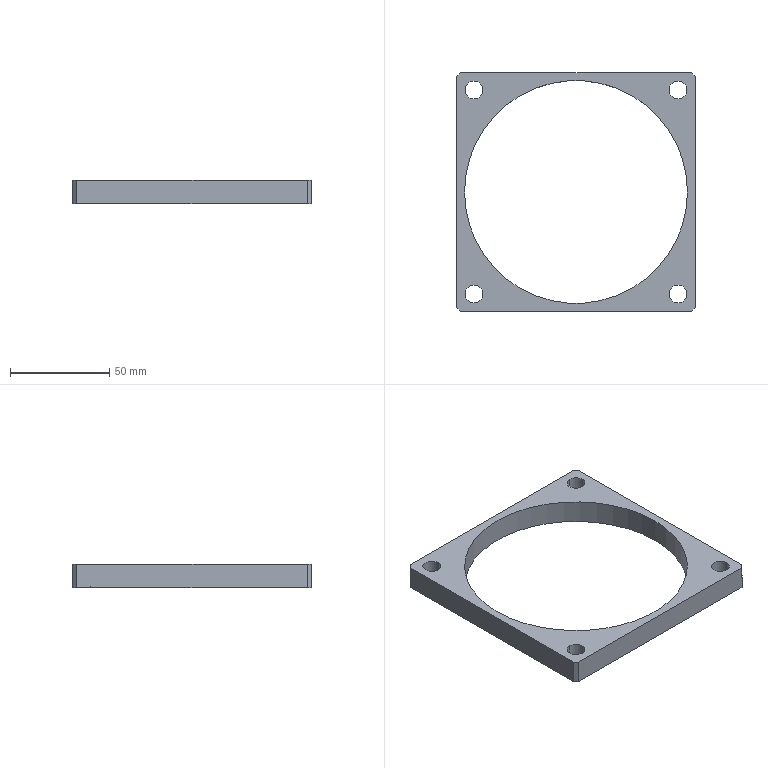Part | SolidWorks | features Chamfer 1, CirPattern 1, Extrusion 1, HoleWzd 1, ICE 1 | 1 solid | 20 faces | box 120 x 120 x 12 mm | volume 51426 mm3 | cylinder 10 | plane 10 | commonest cylinder face diameters 9 x8 112 x2
STEP:
#1=CARTESIAN_POINT('',(51.265,55.765,0.));
#2=VERTEX_POINT('',#1);
#3=CARTESIAN_POINT('',(51.265,46.765,0.));
#4=VERTEX_POINT('',#3);
#5=CARTESIAN_POINT('',(51.265,51.265,0.));
#6=DIRECTION('',(0.,0.,1.));
#7=DIRECTION('',(0.,-1.,0.));
#8=AXIS2_PLACEMENT_3D('',#5,#6,#7);
#9=CIRCLE('',#8,4.5);
#10=EDGE_CURVE('',#2,#4,#9,.T.);
#11=ORIENTED_EDGE('',*,*,#10,.F.);
#12=CARTESIAN_POINT('',(51.265,55.765,12.));
#13=VERTEX_POINT('',#12);
#14=CARTESIAN_POINT('',(51.265,55.765,12.));
#15=DIRECTION('',(0.,0.,1.));
#16=VECTOR('',#15,1000.);
#17=LINE('',#14,#16);
#18=EDGE_CURVE('',#2,#13,#17,.T.);
#19=ORIENTED_EDGE('',*,*,#18,.T.);
#20=CARTESIAN_POINT('',(51.265,46.765,12.));
#21=VERTEX_POINT('',#20);
#22=CARTESIAN_POINT('',(51.265,51.265,12.));
#23=DIRECTION('',(0.,0.,1.));
#24=DIRECTION('',(0.,-1.,0.));
#25=AXIS2_PLACEMENT_3D('',#22,#23,#24);
#26=CIRCLE('',#25,4.5);
#27=EDGE_CURVE('',#13,#21,#26,.T.);
#28=ORIENTED_EDGE('',*,*,#27,.T.);
#29=CARTESIAN_POINT('',(51.265,46.765,12.));
#30=DIRECTION('',(0.,0.,1.));
#31=VECTOR('',#30,1000.);
#32=LINE('',#29,#31);
#33=EDGE_CURVE('',#4,#21,#32,.T.);
#34=ORIENTED_EDGE('',*,*,#33,.F.);
#35=EDGE_LOOP('',(#11,#19,#28,#34));
#36=FACE_OUTER_BOUND('',#35,.T.);
#37=CARTESIAN_POINT('',(51.265,51.265,12.));
#38=DIRECTION('',(0.,0.,1.));
#39=DIRECTION('',(0.,-1.,0.));
#40=AXIS2_PLACEMENT_3D('',#37,#38,#39);
#41=CYLINDRICAL_SURFACE('',#40,4.5);
#42=ADVANCED_FACE('',(#36),#41,.F.);
#43=CARTESIAN_POINT('',(55.765,-51.265,0.));
#44=VERTEX_POINT('',#43);
#45=CARTESIAN_POINT('',(46.765,-51.265,0.));
#46=VERTEX_POINT('',#45);
#47=CARTESIAN_POINT('',(51.265,-51.265,0.));
#48=DIRECTION('',(0.,0.,1.));
#49=DIRECTION('',(-1.,0.,0.));
#50=AXIS2_PLACEMENT_3D('',#47,#48,#49);
#51=CIRCLE('',#50,4.5);
#52=EDGE_CURVE('',#44,#46,#51,.T.);
#53=ORIENTED_EDGE('',*,*,#52,.F.);
#54=CARTESIAN_POINT('',(55.765,-51.265,12.));
#55=VERTEX_POINT('',#54);
#56=CARTESIAN_POINT('',(55.765,-51.265,12.));
#57=DIRECTION('',(0.,0.,1.));
#58=VECTOR('',#57,1000.);
#59=LINE('',#56,#58);
#60=EDGE_CURVE('',#44,#55,#59,.T.);
#61=ORIENTED_EDGE('',*,*,#60,.T.);
#62=CARTESIAN_POINT('',(46.765,-51.265,12.));
#63=VERTEX_POINT('',#62);
#64=CARTESIAN_POINT('',(51.265,-51.265,12.));
#65=DIRECTION('',(0.,0.,1.));
#66=DIRECTION('',(-1.,0.,0.));
#67=AXIS2_PLACEMENT_3D('',#64,#65,#66);
#68=CIRCLE('',#67,4.5);
#69=EDGE_CURVE('',#55,#63,#68,.T.);
#70=ORIENTED_EDGE('',*,*,#69,.T.);
#71=CARTESIAN_POINT('',(46.765,-51.265,12.));
#72=DIRECTION('',(0.,0.,1.));
#73=VECTOR('',#72,1000.);
#74=LINE('',#71,#73);
#75=EDGE_CURVE('',#46,#63,#74,.T.);
#76=ORIENTED_EDGE('',*,*,#75,.F.);
#77=EDGE_LOOP('',(#53,#61,#70,#76));
#78=FACE_OUTER_BOUND('',#77,.T.);
#79=CARTESIAN_POINT('',(51.265,-51.265,12.));
#80=DIRECTION('',(0.,0.,1.));
#81=DIRECTION('',(-1.,0.,0.));
#82=AXIS2_PLACEMENT_3D('',#79,#80,#81);
#83=CYLINDRICAL_SURFACE('',#82,4.5);
#84=ADVANCED_FACE('',(#78),#83,.F.);
#85=CARTESIAN_POINT('',(-51.265,-55.765,0.));
#86=VERTEX_POINT('',#85);
#87=CARTESIAN_POINT('',(-51.265,-46.765,0.));
#88=VERTEX_POINT('',#87);
#89=CARTESIAN_POINT('',(-51.265,-51.265,0.));
#90=DIRECTION('',(0.,0.,1.));
#91=DIRECTION('',(0.,1.,0.));
#92=AXIS2_PLACEMENT_3D('',#89,#90,#91);
#93=CIRCLE('',#92,4.5);
#94=EDGE_CURVE('',#86,#88,#93,.T.);
#95=ORIENTED_EDGE('',*,*,#94,.F.);
#96=CARTESIAN_POINT('',(-51.265,-55.765,12.));
#97=VERTEX_POINT('',#96);
#98=CARTESIAN_POINT('',(-51.265,-55.765,12.));
#99=DIRECTION('',(0.,0.,1.));
#100=VECTOR('',#99,1000.);
#101=LINE('',#98,#100);
#102=EDGE_CURVE('',#86,#97,#101,.T.);
#103=ORIENTED_EDGE('',*,*,#102,.T.);
#104=CARTESIAN_POINT('',(-51.265,-46.765,12.));
#105=VERTEX_POINT('',#104);
#106=CARTESIAN_POINT('',(-51.265,-51.265,12.));
#107=DIRECTION('',(0.,0.,1.));
#108=DIRECTION('',(0.,1.,0.));
#109=AXIS2_PLACEMENT_3D('',#106,#107,#108);
#110=CIRCLE('',#109,4.5);
#111=EDGE_CURVE('',#97,#105,#110,.T.);
#112=ORIENTED_EDGE('',*,*,#111,.T.);
#113=CARTESIAN_POINT('',(-51.265,-46.765,12.));
#114=DIRECTION('',(0.,0.,1.));
#115=VECTOR('',#114,1000.);
#116=LINE('',#113,#115);
#117=EDGE_CURVE('',#88,#105,#116,.T.);
#118=ORIENTED_EDGE('',*,*,#117,.F.);
#119=EDGE_LOOP('',(#95,#103,#112,#118));
#120=FACE_OUTER_BOUND('',#119,.T.);
#121=CARTESIAN_POINT('',(-51.265,-51.265,12.));
#122=DIRECTION('',(0.,0.,1.));
#123=DIRECTION('',(0.,1.,0.));
#124=AXIS2_PLACEMENT_3D('',#121,#122,#123);
#125=CYLINDRICAL_SURFACE('',#124,4.5);
#126=ADVANCED_FACE('',(#120),#125,.F.);
#127=CARTESIAN_POINT('',(-55.765,51.265,0.));
#128=VERTEX_POINT('',#127);
#129=CARTESIAN_POINT('',(-46.765,51.265,0.));
#130=VERTEX_POINT('',#129);
#131=CARTESIAN_POINT('',(-51.265,51.265,0.));
#132=DIRECTION('',(0.,0.,1.));
#133=DIRECTION('',(1.,0.,0.));
#134=AXIS2_PLACEMENT_3D('',#131,#132,#133);
#135=CIRCLE('',#134,4.5);
#136=EDGE_CURVE('',#128,#130,#135,.T.);
#137=ORIENTED_EDGE('',*,*,#136,.F.);
#138=CARTESIAN_POINT('',(-55.765,51.265,12.));
#139=VERTEX_POINT('',#138);
#140=CARTESIAN_POINT('',(-55.765,51.265,12.));
#141=DIRECTION('',(0.,0.,1.));
#142=VECTOR('',#141,1000.);
#143=LINE('',#140,#142);
#144=EDGE_CURVE('',#128,#139,#143,.T.);
#145=ORIENTED_EDGE('',*,*,#144,.T.);
#146=CARTESIAN_POINT('',(-46.765,51.265,12.));
#147=VERTEX_POINT('',#146);
#148=CARTESIAN_POINT('',(-51.265,51.265,12.));
#149=DIRECTION('',(0.,0.,1.));
#150=DIRECTION('',(1.,0.,0.));
#151=AXIS2_PLACEMENT_3D('',#148,#149,#150);
#152=CIRCLE('',#151,4.5);
#153=EDGE_CURVE('',#139,#147,#152,.T.);
#154=ORIENTED_EDGE('',*,*,#153,.T.);
#155=CARTESIAN_POINT('',(-46.765,51.265,12.));
#156=DIRECTION('',(0.,0.,1.));
#157=VECTOR('',#156,1000.);
#158=LINE('',#155,#157);
#159=EDGE_CURVE('',#130,#147,#158,.T.);
#160=ORIENTED_EDGE('',*,*,#159,.F.);
#161=EDGE_LOOP('',(#137,#145,#154,#160));
#162=FACE_OUTER_BOUND('',#161,.T.);
#163=CARTESIAN_POINT('',(-51.265,51.265,12.));
#164=DIRECTION('',(0.,0.,1.));
#165=DIRECTION('',(1.,0.,0.));
#166=AXIS2_PLACEMENT_3D('',#163,#164,#165);
#167=CYLINDRICAL_SURFACE('',#166,4.5);
#168=ADVANCED_FACE('',(#162),#167,.F.);
#169=CARTESIAN_POINT('',(-56.,0.,0.));
#170=VERTEX_POINT('',#169);
#171=CARTESIAN_POINT('',(56.,0.,0.));
#172=VERTEX_POINT('',#171);
#173=CARTESIAN_POINT('',(0.,0.,0.));
#174=DIRECTION('',(0.,0.,1.));
#175=DIRECTION('',(1.,0.,0.));
#176=AXIS2_PLACEMENT_3D('',#173,#174,#175);
#177=CIRCLE('',#176,56.);
#178=EDGE_CURVE('',#170,#172,#177,.T.);
#179=ORIENTED_EDGE('',*,*,#178,.F.);
#180=CARTESIAN_POINT('',(-56.,0.,12.));
#181=VERTEX_POINT('',#180);
#182=CARTESIAN_POINT('',(-56.,0.,0.));
#183=DIRECTION('',(0.,0.,1.));
#184=VECTOR('',#183,1000.);
#185=LINE('',#182,#184);
#186=EDGE_CURVE('',#170,#181,#185,.T.);
#187=ORIENTED_EDGE('',*,*,#186,.T.);
#188=CARTESIAN_POINT('',(56.,0.,12.));
#189=VERTEX_POINT('',#188);
#190=CARTESIAN_POINT('',(0.,0.,12.));
#191=DIRECTION('',(0.,0.,1.));
#192=DIRECTION('',(1.,0.,0.));
#193=AXIS2_PLACEMENT_3D('',#190,#191,#192);
#194=CIRCLE('',#193,56.);
#195=EDGE_CURVE('',#181,#189,#194,.T.);
#196=ORIENTED_EDGE('',*,*,#195,.T.);
#197=CARTESIAN_POINT('',(56.,0.,0.));
#198=DIRECTION('',(0.,0.,1.));
#199=VECTOR('',#198,1000.);
#200=LINE('',#197,#199);
#201=EDGE_CURVE('',#172,#189,#200,.T.);
#202=ORIENTED_EDGE('',*,*,#201,.F.);
#203=EDGE_LOOP('',(#179,#187,#196,#202));
#204=FACE_OUTER_BOUND('',#203,.T.);
#205=CARTESIAN_POINT('',(0.,0.,0.));
#206=DIRECTION('',(0.,0.,1.));
#207=DIRECTION('',(1.,0.,0.));
#208=AXIS2_PLACEMENT_3D('',#205,#206,#207);
#209=CYLINDRICAL_SURFACE('',#208,56.);
#210=ADVANCED_FACE('',(#204),#209,.F.);
#211=CARTESIAN_POINT('',(60.,-58.,0.));
#212=VERTEX_POINT('',#211);
#213=CARTESIAN_POINT('',(60.,58.,0.));
#214=VERTEX_POINT('',#213);
#215=CARTESIAN_POINT('',(60.,60.,0.));
#216=DIRECTION('',(0.,1.,0.));
#217=VECTOR('',#216,1000.);
#218=LINE('',#215,#217);
#219=EDGE_CURVE('',#212,#214,#218,.T.);
#220=ORIENTED_EDGE('',*,*,#219,.T.);
#221=CARTESIAN_POINT('',(60.,58.,12.));
#222=VERTEX_POINT('',#221);
#223=CARTESIAN_POINT('',(60.,58.,12.));
#224=DIRECTION('',(0.,0.,1.));
#225=VECTOR('',#224,1000.);
#226=LINE('',#223,#225);
#227=EDGE_CURVE('',#214,#222,#226,.T.);
#228=ORIENTED_EDGE('',*,*,#227,.T.);
#229=CARTESIAN_POINT('',(60.,-58.,12.));
#230=VERTEX_POINT('',#229);
#231=CARTESIAN_POINT('',(60.,60.,12.));
#232=DIRECTION('',(0.,1.,0.));
#233=VECTOR('',#232,1000.);
#234=LINE('',#231,#233);
#235=EDGE_CURVE('',#230,#222,#234,.T.);
#236=ORIENTED_EDGE('',*,*,#235,.F.);
#237=CARTESIAN_POINT('',(60.,-58.,12.));
#238=DIRECTION('',(0.,0.,-1.));
#239=VECTOR('',#238,1000.);
#240=LINE('',#237,#239);
#241=EDGE_CURVE('',#230,#212,#240,.T.);
#242=ORIENTED_EDGE('',*,*,#241,.T.);
#243=EDGE_LOOP('',(#220,#228,#236,#242));
#244=FACE_OUTER_BOUND('',#243,.T.);
#245=CARTESIAN_POINT('',(60.,60.,12.));
#246=DIRECTION('',(-1.,0.,0.));
#247=DIRECTION('',(0.,-1.,0.));
#248=AXIS2_PLACEMENT_3D('',#245,#246,#247);
#249=PLANE('',#248);
#250=ADVANCED_FACE('',(#244),#249,.F.);
#251=CARTESIAN_POINT('',(58.,60.,12.));
#252=VERTEX_POINT('',#251);
#253=CARTESIAN_POINT('',(-58.,60.,12.));
#254=VERTEX_POINT('',#253);
#255=CARTESIAN_POINT('',(-60.,60.,12.));
#256=DIRECTION('',(-1.,0.,0.));
#257=VECTOR('',#256,1000.);
#258=LINE('',#255,#257);
#259=EDGE_CURVE('',#252,#254,#258,.T.);
#260=ORIENTED_EDGE('',*,*,#259,.F.);
#261=CARTESIAN_POINT('',(58.,60.,0.));
#262=VERTEX_POINT('',#261);
#263=CARTESIAN_POINT('',(58.,60.,12.));
#264=DIRECTION('',(0.,0.,-1.));
#265=VECTOR('',#264,1000.);
#266=LINE('',#263,#265);
#267=EDGE_CURVE('',#252,#262,#266,.T.);
#268=ORIENTED_EDGE('',*,*,#267,.T.);
#269=CARTESIAN_POINT('',(-58.,60.,0.));
#270=VERTEX_POINT('',#269);
#271=CARTESIAN_POINT('',(-60.,60.,0.));
#272=DIRECTION('',(-1.,0.,0.));
#273=VECTOR('',#272,1000.);
#274=LINE('',#271,#273);
#275=EDGE_CURVE('',#262,#270,#274,.T.);
#276=ORIENTED_EDGE('',*,*,#275,.T.);
#277=CARTESIAN_POINT('',(-58.,60.,12.));
#278=DIRECTION('',(0.,0.,1.));
#279=VECTOR('',#278,1000.);
#280=LINE('',#277,#279);
#281=EDGE_CURVE('',#270,#254,#280,.T.);
#282=ORIENTED_EDGE('',*,*,#281,.T.);
#283=EDGE_LOOP('',(#260,#268,#276,#282));
#284=FACE_OUTER_BOUND('',#283,.T.);
#285=CARTESIAN_POINT('',(-60.,60.,12.));
#286=DIRECTION('',(0.,-1.,0.));
#287=DIRECTION('',(0.,0.,-1.));
#288=AXIS2_PLACEMENT_3D('',#285,#286,#287);
#289=PLANE('',#288);
#290=ADVANCED_FACE('',(#284),#289,.F.);
#291=CARTESIAN_POINT('',(-60.,58.,0.));
#292=VERTEX_POINT('',#291);
#293=CARTESIAN_POINT('',(-60.,-58.,0.));
#294=VERTEX_POINT('',#293);
#295=CARTESIAN_POINT('',(-60.,60.,0.));
#296=DIRECTION('',(0.,-1.,0.));
#297=VECTOR('',#296,1000.);
#298=LINE('',#295,#297);
#299=EDGE_CURVE('',#292,#294,#298,.T.);
#300=ORIENTED_EDGE('',*,*,#299,.T.);
#301=CARTESIAN_POINT('',(-60.,-58.,12.));
#302=VERTEX_POINT('',#301);
#303=CARTESIAN_POINT('',(-60.,-58.,12.));
#304=DIRECTION('',(0.,0.,1.));
#305=VECTOR('',#304,1000.);
#306=LINE('',#303,#305);
#307=EDGE_CURVE('',#294,#302,#306,.T.);
#308=ORIENTED_EDGE('',*,*,#307,.T.);
#309=CARTESIAN_POINT('',(-60.,58.,12.));
#310=VERTEX_POINT('',#309);
#311=CARTESIAN_POINT('',(-60.,60.,12.));
#312=DIRECTION('',(0.,-1.,0.));
#313=VECTOR('',#312,1000.);
#314=LINE('',#311,#313);
#315=EDGE_CURVE('',#310,#302,#314,.T.);
#316=ORIENTED_EDGE('',*,*,#315,.F.);
#317=CARTESIAN_POINT('',(-60.,58.,12.));
#318=DIRECTION('',(0.,0.,-1.));
#319=VECTOR('',#318,1000.);
#320=LINE('',#317,#319);
#321=EDGE_CURVE('',#310,#292,#320,.T.);
#322=ORIENTED_EDGE('',*,*,#321,.T.);
#323=EDGE_LOOP('',(#300,#308,#316,#322));
#324=FACE_OUTER_BOUND('',#323,.T.);
#325=CARTESIAN_POINT('',(-60.,60.,12.));
#326=DIRECTION('',(1.,0.,0.));
#327=DIRECTION('',(0.,1.,0.));
#328=AXIS2_PLACEMENT_3D('',#325,#326,#327);
#329=PLANE('',#328);
#330=ADVANCED_FACE('',(#324),#329,.F.);
#331=CARTESIAN_POINT('',(-58.,-60.,0.));
#332=VERTEX_POINT('',#331);
#333=CARTESIAN_POINT('',(58.,-60.,0.));
#334=VERTEX_POINT('',#333);
#335=CARTESIAN_POINT('',(-60.,-60.,0.));
#336=DIRECTION('',(1.,0.,0.));
#337=VECTOR('',#336,1000.);
#338=LINE('',#335,#337);
#339=EDGE_CURVE('',#332,#334,#338,.T.);
#340=ORIENTED_EDGE('',*,*,#339,.T.);
#341=CARTESIAN_POINT('',(58.,-60.,12.));
#342=VERTEX_POINT('',#341);
#343=CARTESIAN_POINT('',(58.,-60.,12.));
#344=DIRECTION('',(0.,0.,1.));
#345=VECTOR('',#344,1000.);
#346=LINE('',#343,#345);
#347=EDGE_CURVE('',#334,#342,#346,.T.);
#348=ORIENTED_EDGE('',*,*,#347,.T.);
#349=CARTESIAN_POINT('',(-58.,-60.,12.));
#350=VERTEX_POINT('',#349);
#351=CARTESIAN_POINT('',(-60.,-60.,12.));
#352=DIRECTION('',(1.,0.,0.));
#353=VECTOR('',#352,1000.);
#354=LINE('',#351,#353);
#355=EDGE_CURVE('',#350,#342,#354,.T.);
#356=ORIENTED_EDGE('',*,*,#355,.F.);
#357=CARTESIAN_POINT('',(-58.,-60.,12.));
#358=DIRECTION('',(0.,0.,-1.));
#359=VECTOR('',#358,1000.);
#360=LINE('',#357,#359);
#361=EDGE_CURVE('',#350,#332,#360,.T.);
#362=ORIENTED_EDGE('',*,*,#361,.T.);
#363=EDGE_LOOP('',(#340,#348,#356,#362));
#364=FACE_OUTER_BOUND('',#363,.T.);
#365=CARTESIAN_POINT('',(-60.,-60.,12.));
#366=DIRECTION('',(0.,1.,0.));
#367=DIRECTION('',(0.,0.,1.));
#368=AXIS2_PLACEMENT_3D('',#365,#366,#367);
#369=PLANE('',#368);
#370=ADVANCED_FACE('',(#364),#369,.F.);
#371=CARTESIAN_POINT('',(51.265,51.265,12.));
#372=DIRECTION('',(0.,0.,1.));
#373=DIRECTION('',(0.,-1.,0.));
#374=AXIS2_PLACEMENT_3D('',#371,#372,#373);
#375=CIRCLE('',#374,4.5);
#376=EDGE_CURVE('',#21,#13,#375,.T.);
#377=ORIENTED_EDGE('',*,*,#376,.F.);
#378=ORIENTED_EDGE('',*,*,#27,.F.);
#379=EDGE_LOOP('',(#377,#378));
#380=FACE_BOUND('',#379,.T.);
#381=CARTESIAN_POINT('',(51.265,-51.265,12.));
#382=DIRECTION('',(0.,0.,1.));
#383=DIRECTION('',(-1.,0.,0.));
#384=AXIS2_PLACEMENT_3D('',#381,#382,#383);
#385=CIRCLE('',#384,4.5);
#386=EDGE_CURVE('',#63,#55,#385,.T.);
#387=ORIENTED_EDGE('',*,*,#386,.F.);
#388=ORIENTED_EDGE('',*,*,#69,.F.);
#389=EDGE_LOOP('',(#387,#388));
#390=FACE_BOUND('',#389,.T.);
#391=CARTESIAN_POINT('',(-51.265,-51.265,12.));
#392=DIRECTION('',(0.,0.,1.));
#393=DIRECTION('',(0.,1.,0.));
#394=AXIS2_PLACEMENT_3D('',#391,#392,#393);
#395=CIRCLE('',#394,4.5);
#396=EDGE_CURVE('',#105,#97,#395,.T.);
#397=ORIENTED_EDGE('',*,*,#396,.F.);
#398=ORIENTED_EDGE('',*,*,#111,.F.);
#399=EDGE_LOOP('',(#397,#398));
#400=FACE_BOUND('',#399,.T.);
#401=CARTESIAN_POINT('',(-51.265,51.265,12.));
#402=DIRECTION('',(0.,0.,1.));
#403=DIRECTION('',(1.,0.,0.));
#404=AXIS2_PLACEMENT_3D('',#401,#402,#403);
#405=CIRCLE('',#404,4.5);
#406=EDGE_CURVE('',#147,#139,#405,.T.);
#407=ORIENTED_EDGE('',*,*,#406,.F.);
#408=ORIENTED_EDGE('',*,*,#153,.F.);
#409=EDGE_LOOP('',(#407,#408));
#410=FACE_BOUND('',#409,.T.);
#411=CARTESIAN_POINT('',(0.,0.,12.));
#412=DIRECTION('',(0.,0.,1.));
#413=DIRECTION('',(1.,0.,0.));
#414=AXIS2_PLACEMENT_3D('',#411,#412,#413);
#415=CIRCLE('',#414,56.);
#416=EDGE_CURVE('',#189,#181,#415,.T.);
#417=ORIENTED_EDGE('',*,*,#416,.F.);
#418=ORIENTED_EDGE('',*,*,#195,.F.);
#419=EDGE_LOOP('',(#417,#418));
#420=FACE_BOUND('',#419,.T.);
#421=ORIENTED_EDGE('',*,*,#235,.T.);
#422=CARTESIAN_POINT('',(119.,-1.,12.));
#423=DIRECTION('',(-0.7071,0.7071,0.));
#424=VECTOR('',#423,1000.);
#425=LINE('',#422,#424);
#426=EDGE_CURVE('',#222,#252,#425,.T.);
#427=ORIENTED_EDGE('',*,*,#426,.T.);
#428=ORIENTED_EDGE('',*,*,#259,.T.);
#429=CARTESIAN_POINT('',(-59.,59.,12.));
#430=DIRECTION('',(-0.7071,-0.7071,0.));
#431=VECTOR('',#430,1000.);
#432=LINE('',#429,#431);
#433=EDGE_CURVE('',#254,#310,#432,.T.);
#434=ORIENTED_EDGE('',*,*,#433,.T.);
#435=ORIENTED_EDGE('',*,*,#315,.T.);
#436=CARTESIAN_POINT('',(1.,-119.,12.));
#437=DIRECTION('',(0.7071,-0.7071,0.));
#438=VECTOR('',#437,1000.);
#439=LINE('',#436,#438);
#440=EDGE_CURVE('',#302,#350,#439,.T.);
#441=ORIENTED_EDGE('',*,*,#440,.T.);
#442=ORIENTED_EDGE('',*,*,#355,.T.);
#443=CARTESIAN_POINT('',(59.,-59.,12.));
#444=DIRECTION('',(0.7071,0.7071,0.));
#445=VECTOR('',#444,1000.);
#446=LINE('',#443,#445);
#447=EDGE_CURVE('',#342,#230,#446,.T.);
#448=ORIENTED_EDGE('',*,*,#447,.T.);
#449=EDGE_LOOP('',(#421,#427,#428,#434,#435,#441,#442,#448));
#450=FACE_OUTER_BOUND('',#449,.T.);
#451=CARTESIAN_POINT('',(60.,-60.,12.));
#452=DIRECTION('',(0.,0.,1.));
#453=DIRECTION('',(1.,0.,0.));
#454=AXIS2_PLACEMENT_3D('',#451,#452,#453);
#455=PLANE('',#454);
#456=ADVANCED_FACE('',(#380,#390,#400,#410,#420,#450),#455,.T.);
#457=CARTESIAN_POINT('',(51.265,51.265,0.));
#458=DIRECTION('',(0.,0.,1.));
#459=DIRECTION('',(0.,-1.,0.));
#460=AXIS2_PLACEMENT_3D('',#457,#458,#459);
#461=CIRCLE('',#460,4.5);
#462=EDGE_CURVE('',#4,#2,#461,.T.);
#463=ORIENTED_EDGE('',*,*,#462,.T.);
#464=ORIENTED_EDGE('',*,*,#10,.T.);
#465=EDGE_LOOP('',(#463,#464));
#466=FACE_BOUND('',#465,.T.);
#467=CARTESIAN_POINT('',(51.265,-51.265,0.));
#468=DIRECTION('',(0.,0.,1.));
#469=DIRECTION('',(-1.,0.,0.));
#470=AXIS2_PLACEMENT_3D('',#467,#468,#469);
#471=CIRCLE('',#470,4.5);
#472=EDGE_CURVE('',#46,#44,#471,.T.);
#473=ORIENTED_EDGE('',*,*,#472,.T.);
#474=ORIENTED_EDGE('',*,*,#52,.T.);
#475=EDGE_LOOP('',(#473,#474));
#476=FACE_BOUND('',#475,.T.);
#477=CARTESIAN_POINT('',(-51.265,-51.265,0.));
#478=DIRECTION('',(0.,0.,1.));
#479=DIRECTION('',(0.,1.,0.));
#480=AXIS2_PLACEMENT_3D('',#477,#478,#479);
#481=CIRCLE('',#480,4.5);
#482=EDGE_CURVE('',#88,#86,#481,.T.);
#483=ORIENTED_EDGE('',*,*,#482,.T.);
#484=ORIENTED_EDGE('',*,*,#94,.T.);
#485=EDGE_LOOP('',(#483,#484));
#486=FACE_BOUND('',#485,.T.);
#487=CARTESIAN_POINT('',(-51.265,51.265,0.));
#488=DIRECTION('',(0.,0.,1.));
#489=DIRECTION('',(1.,0.,0.));
#490=AXIS2_PLACEMENT_3D('',#487,#488,#489);
#491=CIRCLE('',#490,4.5);
#492=EDGE_CURVE('',#130,#128,#491,.T.);
#493=ORIENTED_EDGE('',*,*,#492,.T.);
#494=ORIENTED_EDGE('',*,*,#136,.T.);
#495=EDGE_LOOP('',(#493,#494));
#496=FACE_BOUND('',#495,.T.);
#497=CARTESIAN_POINT('',(0.,0.,0.));
#498=DIRECTION('',(0.,0.,1.));
#499=DIRECTION('',(1.,0.,0.));
#500=AXIS2_PLACEMENT_3D('',#497,#498,#499);
#501=CIRCLE('',#500,56.);
#502=EDGE_CURVE('',#172,#170,#501,.T.);
#503=ORIENTED_EDGE('',*,*,#502,.T.);
#504=ORIENTED_EDGE('',*,*,#178,.T.);
#505=EDGE_LOOP('',(#503,#504));
#506=FACE_BOUND('',#505,.T.);
#507=ORIENTED_EDGE('',*,*,#275,.F.);
#508=CARTESIAN_POINT('',(58.,60.,0.));
#509=DIRECTION('',(0.7071,-0.7071,0.));
#510=VECTOR('',#509,1000.);
#511=LINE('',#508,#510);
#512=EDGE_CURVE('',#262,#214,#511,.T.);
#513=ORIENTED_EDGE('',*,*,#512,.T.);
#514=ORIENTED_EDGE('',*,*,#219,.F.);
#515=CARTESIAN_POINT('',(60.,-58.,0.));
#516=DIRECTION('',(-0.7071,-0.7071,0.));
#517=VECTOR('',#516,1000.);
#518=LINE('',#515,#517);
#519=EDGE_CURVE('',#212,#334,#518,.T.);
#520=ORIENTED_EDGE('',*,*,#519,.T.);
#521=ORIENTED_EDGE('',*,*,#339,.F.);
#522=CARTESIAN_POINT('',(-58.,-60.,0.));
#523=DIRECTION('',(-0.7071,0.7071,0.));
#524=VECTOR('',#523,1000.);
#525=LINE('',#522,#524);
#526=EDGE_CURVE('',#332,#294,#525,.T.);
#527=ORIENTED_EDGE('',*,*,#526,.T.);
#528=ORIENTED_EDGE('',*,*,#299,.F.);
#529=CARTESIAN_POINT('',(-60.,58.,0.));
#530=DIRECTION('',(0.7071,0.7071,0.));
#531=VECTOR('',#530,1000.);
#532=LINE('',#529,#531);
#533=EDGE_CURVE('',#292,#270,#532,.T.);
#534=ORIENTED_EDGE('',*,*,#533,.T.);
#535=EDGE_LOOP('',(#507,#513,#514,#520,#521,#527,#528,#534));
#536=FACE_OUTER_BOUND('',#535,.T.);
#537=CARTESIAN_POINT('',(60.,-60.,0.));
#538=DIRECTION('',(0.,0.,1.));
#539=DIRECTION('',(1.,0.,0.));
#540=AXIS2_PLACEMENT_3D('',#537,#538,#539);
#541=PLANE('',#540);
#542=ADVANCED_FACE('',(#466,#476,#486,#496,#506,#536),#541,.F.);
#543=ORIENTED_EDGE('',*,*,#186,.F.);
#544=ORIENTED_EDGE('',*,*,#502,.F.);
#545=ORIENTED_EDGE('',*,*,#201,.T.);
#546=ORIENTED_EDGE('',*,*,#416,.T.);
#547=EDGE_LOOP('',(#543,#544,#545,#546));
#548=FACE_OUTER_BOUND('',#547,.T.);
#549=CARTESIAN_POINT('',(0.,0.,0.));
#550=DIRECTION('',(0.,0.,1.));
#551=DIRECTION('',(1.,0.,0.));
#552=AXIS2_PLACEMENT_3D('',#549,#550,#551);
#553=CYLINDRICAL_SURFACE('',#552,56.);
#554=ADVANCED_FACE('',(#548),#553,.F.);
#555=ORIENTED_EDGE('',*,*,#144,.F.);
#556=ORIENTED_EDGE('',*,*,#492,.F.);
#557=ORIENTED_EDGE('',*,*,#159,.T.);
#558=ORIENTED_EDGE('',*,*,#406,.T.);
#559=EDGE_LOOP('',(#555,#556,#557,#558));
#560=FACE_OUTER_BOUND('',#559,.T.);
#561=CARTESIAN_POINT('',(-51.265,51.265,12.));
#562=DIRECTION('',(0.,0.,1.));
#563=DIRECTION('',(1.,0.,0.));
#564=AXIS2_PLACEMENT_3D('',#561,#562,#563);
#565=CYLINDRICAL_SURFACE('',#564,4.5);
#566=ADVANCED_FACE('',(#560),#565,.F.);
#567=ORIENTED_EDGE('',*,*,#102,.F.);
#568=ORIENTED_EDGE('',*,*,#482,.F.);
#569=ORIENTED_EDGE('',*,*,#117,.T.);
#570=ORIENTED_EDGE('',*,*,#396,.T.);
#571=EDGE_LOOP('',(#567,#568,#569,#570));
#572=FACE_OUTER_BOUND('',#571,.T.);
#573=CARTESIAN_POINT('',(-51.265,-51.265,12.));
#574=DIRECTION('',(0.,0.,1.));
#575=DIRECTION('',(0.,1.,0.));
#576=AXIS2_PLACEMENT_3D('',#573,#574,#575);
#577=CYLINDRICAL_SURFACE('',#576,4.5);
#578=ADVANCED_FACE('',(#572),#577,.F.);
#579=ORIENTED_EDGE('',*,*,#60,.F.);
#580=ORIENTED_EDGE('',*,*,#472,.F.);
#581=ORIENTED_EDGE('',*,*,#75,.T.);
#582=ORIENTED_EDGE('',*,*,#386,.T.);
#583=EDGE_LOOP('',(#579,#580,#581,#582));
#584=FACE_OUTER_BOUND('',#583,.T.);
#585=CARTESIAN_POINT('',(51.265,-51.265,12.));
#586=DIRECTION('',(0.,0.,1.));
#587=DIRECTION('',(-1.,0.,0.));
#588=AXIS2_PLACEMENT_3D('',#585,#586,#587);
#589=CYLINDRICAL_SURFACE('',#588,4.5);
#590=ADVANCED_FACE('',(#584),#589,.F.);
#591=ORIENTED_EDGE('',*,*,#18,.F.);
#592=ORIENTED_EDGE('',*,*,#462,.F.);
#593=ORIENTED_EDGE('',*,*,#33,.T.);
#594=ORIENTED_EDGE('',*,*,#376,.T.);
#595=EDGE_LOOP('',(#591,#592,#593,#594));
#596=FACE_OUTER_BOUND('',#595,.T.);
#597=CARTESIAN_POINT('',(51.265,51.265,12.));
#598=DIRECTION('',(0.,0.,1.));
#599=DIRECTION('',(0.,-1.,0.));
#600=AXIS2_PLACEMENT_3D('',#597,#598,#599);
#601=CYLINDRICAL_SURFACE('',#600,4.5);
#602=ADVANCED_FACE('',(#596),#601,.F.);
#603=ORIENTED_EDGE('',*,*,#426,.F.);
#604=ORIENTED_EDGE('',*,*,#227,.F.);
#605=ORIENTED_EDGE('',*,*,#512,.F.);
#606=ORIENTED_EDGE('',*,*,#267,.F.);
#607=EDGE_LOOP('',(#603,#604,#605,#606));
#608=FACE_OUTER_BOUND('',#607,.T.);
#609=CARTESIAN_POINT('',(58.,60.,12.));
#610=DIRECTION('',(-0.7071,-0.7071,0.));
#611=DIRECTION('',(0.7071,-0.7071,0.));
#612=AXIS2_PLACEMENT_3D('',#609,#610,#611);
#613=PLANE('',#612);
#614=ADVANCED_FACE('',(#608),#613,.F.);
#615=ORIENTED_EDGE('',*,*,#447,.F.);
#616=ORIENTED_EDGE('',*,*,#347,.F.);
#617=ORIENTED_EDGE('',*,*,#519,.F.);
#618=ORIENTED_EDGE('',*,*,#241,.F.);
#619=EDGE_LOOP('',(#615,#616,#617,#618));
#620=FACE_OUTER_BOUND('',#619,.T.);
#621=CARTESIAN_POINT('',(60.,-58.,12.));
#622=DIRECTION('',(-0.7071,0.7071,0.));
#623=DIRECTION('',(-0.7071,-0.7071,0.));
#624=AXIS2_PLACEMENT_3D('',#621,#622,#623);
#625=PLANE('',#624);
#626=ADVANCED_FACE('',(#620),#625,.F.);
#627=ORIENTED_EDGE('',*,*,#440,.F.);
#628=ORIENTED_EDGE('',*,*,#307,.F.);
#629=ORIENTED_EDGE('',*,*,#526,.F.);
#630=ORIENTED_EDGE('',*,*,#361,.F.);
#631=EDGE_LOOP('',(#627,#628,#629,#630));
#632=FACE_OUTER_BOUND('',#631,.T.);
#633=CARTESIAN_POINT('',(-58.,-60.,12.));
#634=DIRECTION('',(0.7071,0.7071,0.));
#635=DIRECTION('',(-0.7071,0.7071,0.));
#636=AXIS2_PLACEMENT_3D('',#633,#634,#635);
#637=PLANE('',#636);
#638=ADVANCED_FACE('',(#632),#637,.F.);
#639=ORIENTED_EDGE('',*,*,#433,.F.);
#640=ORIENTED_EDGE('',*,*,#281,.F.);
#641=ORIENTED_EDGE('',*,*,#533,.F.);
#642=ORIENTED_EDGE('',*,*,#321,.F.);
#643=EDGE_LOOP('',(#639,#640,#641,#642));
#644=FACE_OUTER_BOUND('',#643,.T.);
#645=CARTESIAN_POINT('',(-60.,58.,12.));
#646=DIRECTION('',(0.7071,-0.7071,0.));
#647=DIRECTION('',(0.7071,0.7071,0.));
#648=AXIS2_PLACEMENT_3D('',#645,#646,#647);
#649=PLANE('',#648);
#650=ADVANCED_FACE('',(#644),#649,.F.);
#651=CLOSED_SHELL('',(#42,#84,#126,#168,#210,#250,#290,#330,#370,#456,#542,#554,#566,#578,#590,#602,#614,#626,#638,#650));
#652=MANIFOLD_SOLID_BREP('',#651);
#653=CARTESIAN_POINT('',(0.,0.,0.));
#654=DIRECTION('',(0.,0.,1.));
#655=DIRECTION('',(1.,0.,0.));
#656=AXIS2_PLACEMENT_3D('',#653,#654,#655);
#657=(LENGTH_UNIT()NAMED_UNIT(*)SI_UNIT(.MILLI.,.METRE.));
#658=UNCERTAINTY_MEASURE_WITH_UNIT(LENGTH_MEASURE(0.00001),#657,'','');
#659=(NAMED_UNIT(*)PLANE_ANGLE_UNIT()SI_UNIT($,.RADIAN.));
#660=(NAMED_UNIT(*)SI_UNIT($,.STERADIAN.)SOLID_ANGLE_UNIT());
#661=(GEOMETRIC_REPRESENTATION_CONTEXT(3)GLOBAL_UNCERTAINTY_ASSIGNED_CONTEXT((#658))GLOBAL_UNIT_ASSIGNED_CONTEXT((#657,#659,#660))REPRESENTATION_CONTEXT('',''));
#662=ADVANCED_BREP_SHAPE_REPRESENTATION('',(#652,#656),#661);